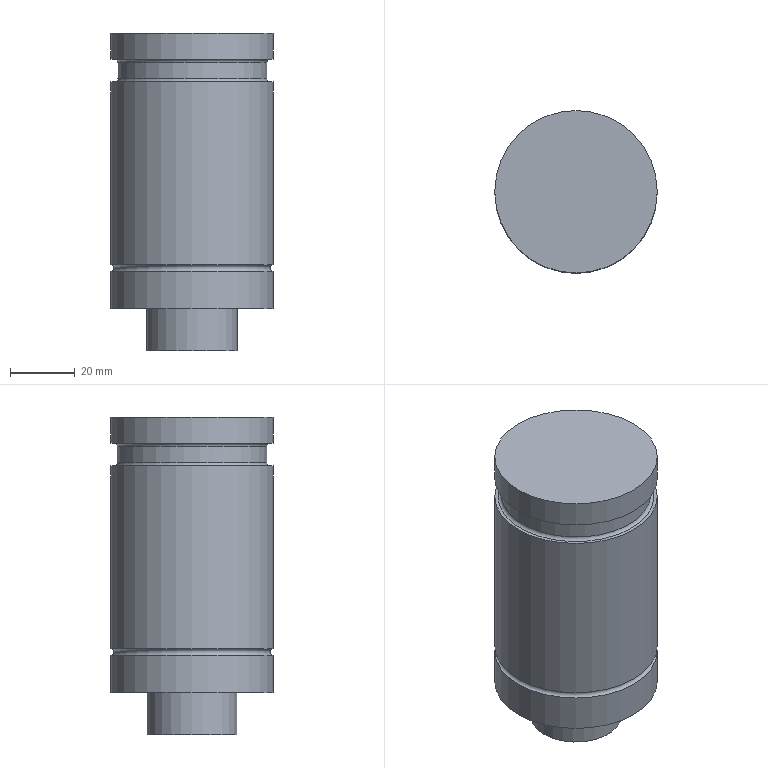Part | NX | features solid 2 | 1 solid | 13 faces | box 50.2 x 50.2 x 98 mm | volume 173939 mm3 | cylinder 5 | plane 5 | torus 3 | commonest cylinder face diameters 50.2 x3 28 x1 46.2 x1
STEP:
#1=CARTESIAN_POINT('',(40.1,-380.,248.5));
#2=VERTEX_POINT('',#1);
#3=CARTESIAN_POINT('',(15.,-380.,248.5));
#4=DIRECTION('',(0.,0.,1.));
#5=DIRECTION('',(1.,0.,0.));
#6=AXIS2_PLACEMENT_3D('',#3,#4,#5);
#7=CIRCLE('',#6,25.1);
#8=EDGE_CURVE('',#2,#2,#7,.T.);
#9=ORIENTED_EDGE('',*,*,#8,.T.);
#10=EDGE_LOOP('',(#9));
#11=FACE_BOUND('',#10,.T.);
#12=CARTESIAN_POINT('',(-10.1,-380.,305.));
#13=VERTEX_POINT('',#12);
#14=CARTESIAN_POINT('',(15.,-380.,305.));
#15=DIRECTION('',(0.,0.,-1.));
#16=DIRECTION('',(-1.,0.,0.));
#17=AXIS2_PLACEMENT_3D('',#14,#15,#16);
#18=CIRCLE('',#17,25.1);
#19=EDGE_CURVE('',#13,#13,#18,.T.);
#20=ORIENTED_EDGE('',*,*,#19,.T.);
#21=EDGE_LOOP('',(#20));
#22=FACE_BOUND('',#21,.T.);
#23=CARTESIAN_POINT('',(15.,-380.,235.));
#24=DIRECTION('',(0.,0.,1.));
#25=DIRECTION('',(1.,0.,0.));
#26=AXIS2_PLACEMENT_3D('',#23,#24,#25);
#27=CYLINDRICAL_SURFACE('',#26,25.1);
#28=ADVANCED_FACE('',(#11,#22),#27,.T.);
#29=CARTESIAN_POINT('',(1.,-380.,235.));
#30=VERTEX_POINT('',#29);
#31=CARTESIAN_POINT('',(15.,-380.,235.));
#32=DIRECTION('',(0.,0.,-1.));
#33=DIRECTION('',(-1.,0.,0.));
#34=AXIS2_PLACEMENT_3D('',#31,#32,#33);
#35=CIRCLE('',#34,14.);
#36=EDGE_CURVE('',#30,#30,#35,.T.);
#37=ORIENTED_EDGE('',*,*,#36,.F.);
#38=EDGE_LOOP('',(#37));
#39=FACE_BOUND('',#38,.T.);
#40=CARTESIAN_POINT('',(40.1,-380.,235.));
#41=VERTEX_POINT('',#40);
#42=CARTESIAN_POINT('',(15.,-380.,235.));
#43=DIRECTION('',(0.,0.,1.));
#44=DIRECTION('',(1.,0.,0.));
#45=AXIS2_PLACEMENT_3D('',#42,#43,#44);
#46=CIRCLE('',#45,25.1);
#47=EDGE_CURVE('',#41,#41,#46,.T.);
#48=ORIENTED_EDGE('',*,*,#47,.F.);
#49=EDGE_LOOP('',(#48));
#50=FACE_BOUND('',#49,.T.);
#51=CARTESIAN_POINT('',(15.,-380.,235.));
#52=DIRECTION('',(0.,0.,-1.));
#53=DIRECTION('',(-1.,0.,0.));
#54=AXIS2_PLACEMENT_3D('',#51,#52,#53);
#55=PLANE('',#54);
#56=ADVANCED_FACE('',(#39,#50),#55,.T.);
#57=CARTESIAN_POINT('',(40.1,-380.,246.5));
#58=VERTEX_POINT('',#57);
#59=CARTESIAN_POINT('',(15.,-380.,246.5));
#60=DIRECTION('',(0.,0.,1.));
#61=DIRECTION('',(1.,0.,0.));
#62=AXIS2_PLACEMENT_3D('',#59,#60,#61);
#63=CIRCLE('',#62,25.1);
#64=EDGE_CURVE('',#58,#58,#63,.T.);
#65=ORIENTED_EDGE('',*,*,#64,.F.);
#66=EDGE_LOOP('',(#65));
#67=FACE_BOUND('',#66,.T.);
#68=ORIENTED_EDGE('',*,*,#47,.T.);
#69=EDGE_LOOP('',(#68));
#70=FACE_BOUND('',#69,.T.);
#71=CARTESIAN_POINT('',(15.,-380.,235.));
#72=DIRECTION('',(0.,0.,1.));
#73=DIRECTION('',(1.,0.,0.));
#74=AXIS2_PLACEMENT_3D('',#71,#72,#73);
#75=CYLINDRICAL_SURFACE('',#74,25.1);
#76=ADVANCED_FACE('',(#67,#70),#75,.T.);
#77=CARTESIAN_POINT('',(29.,-380.,222.));
#78=VERTEX_POINT('',#77);
#79=CARTESIAN_POINT('',(15.,-380.,222.));
#80=DIRECTION('',(0.,0.,1.));
#81=DIRECTION('',(1.,0.,0.));
#82=AXIS2_PLACEMENT_3D('',#79,#80,#81);
#83=CIRCLE('',#82,14.);
#84=EDGE_CURVE('',#78,#78,#83,.T.);
#85=ORIENTED_EDGE('',*,*,#84,.F.);
#86=EDGE_LOOP('',(#85));
#87=FACE_BOUND('',#86,.T.);
#88=CARTESIAN_POINT('',(15.,-380.,222.));
#89=DIRECTION('',(0.,0.,-1.));
#90=DIRECTION('',(-1.,0.,0.));
#91=AXIS2_PLACEMENT_3D('',#88,#89,#90);
#92=PLANE('',#91);
#93=ADVANCED_FACE('',(#87),#92,.T.);
#94=ORIENTED_EDGE('',*,*,#84,.T.);
#95=EDGE_LOOP('',(#94));
#96=FACE_BOUND('',#95,.T.);
#97=ORIENTED_EDGE('',*,*,#36,.T.);
#98=EDGE_LOOP('',(#97));
#99=FACE_BOUND('',#98,.T.);
#100=CARTESIAN_POINT('',(15.,-380.,235.));
#101=DIRECTION('',(0.,0.,-1.));
#102=DIRECTION('',(-1.,0.,0.));
#103=AXIS2_PLACEMENT_3D('',#100,#101,#102);
#104=CYLINDRICAL_SURFACE('',#103,14.);
#105=ADVANCED_FACE('',(#96,#99),#104,.T.);
#106=ORIENTED_EDGE('',*,*,#8,.F.);
#107=EDGE_LOOP('',(#106));
#108=FACE_BOUND('',#107,.T.);
#109=ORIENTED_EDGE('',*,*,#64,.T.);
#110=EDGE_LOOP('',(#109));
#111=FACE_BOUND('',#110,.T.);
#112=CARTESIAN_POINT('',(15.,-380.,247.5));
#113=DIRECTION('',(0.,0.,-1.));
#114=DIRECTION('',(-1.,0.,0.));
#115=AXIS2_PLACEMENT_3D('',#112,#113,#114);
#116=TOROIDAL_SURFACE('',#115,25.1,1.);
#117=ADVANCED_FACE('',(#108,#111),#116,.F.);
#118=CARTESIAN_POINT('',(39.1,-380.,305.));
#119=VERTEX_POINT('',#118);
#120=CARTESIAN_POINT('',(15.,-380.,305.));
#121=DIRECTION('',(0.,0.,1.));
#122=DIRECTION('',(1.,0.,0.));
#123=AXIS2_PLACEMENT_3D('',#120,#121,#122);
#124=CIRCLE('',#123,24.1);
#125=EDGE_CURVE('',#119,#119,#124,.F.);
#126=ORIENTED_EDGE('',*,*,#125,.T.);
#127=EDGE_LOOP('',(#126));
#128=FACE_BOUND('',#127,.T.);
#129=ORIENTED_EDGE('',*,*,#19,.F.);
#130=EDGE_LOOP('',(#129));
#131=FACE_BOUND('',#130,.T.);
#132=CARTESIAN_POINT('',(15.,-380.,305.));
#133=DIRECTION('',(0.,0.,1.));
#134=DIRECTION('',(1.,0.,0.));
#135=AXIS2_PLACEMENT_3D('',#132,#133,#134);
#136=PLANE('',#135);
#137=ADVANCED_FACE('',(#128,#131),#136,.T.);
#138=CARTESIAN_POINT('',(39.1,-380.,312.));
#139=VERTEX_POINT('',#138);
#140=CARTESIAN_POINT('',(15.,-380.,312.));
#141=DIRECTION('',(0.,0.,1.));
#142=DIRECTION('',(1.,0.,0.));
#143=AXIS2_PLACEMENT_3D('',#140,#141,#142);
#144=CIRCLE('',#143,24.1);
#145=EDGE_CURVE('',#139,#139,#144,.T.);
#146=ORIENTED_EDGE('',*,*,#145,.T.);
#147=EDGE_LOOP('',(#146));
#148=FACE_BOUND('',#147,.T.);
#149=CARTESIAN_POINT('',(-10.1,-380.,312.));
#150=VERTEX_POINT('',#149);
#151=CARTESIAN_POINT('',(15.,-380.,312.));
#152=DIRECTION('',(0.,0.,-1.));
#153=DIRECTION('',(-1.,0.,0.));
#154=AXIS2_PLACEMENT_3D('',#151,#152,#153);
#155=CIRCLE('',#154,25.1);
#156=EDGE_CURVE('',#150,#150,#155,.T.);
#157=ORIENTED_EDGE('',*,*,#156,.T.);
#158=EDGE_LOOP('',(#157));
#159=FACE_BOUND('',#158,.T.);
#160=CARTESIAN_POINT('',(15.,-380.,312.));
#161=DIRECTION('',(0.,0.,1.));
#162=DIRECTION('',(1.,0.,0.));
#163=AXIS2_PLACEMENT_3D('',#160,#161,#162);
#164=PLANE('',#163);
#165=ADVANCED_FACE('',(#148,#159),#164,.F.);
#166=CARTESIAN_POINT('',(38.1,-380.,306.));
#167=VERTEX_POINT('',#166);
#168=CARTESIAN_POINT('',(15.,-380.,306.));
#169=DIRECTION('',(0.,0.,1.));
#170=DIRECTION('',(1.,0.,0.));
#171=AXIS2_PLACEMENT_3D('',#168,#169,#170);
#172=CIRCLE('',#171,23.1);
#173=EDGE_CURVE('',#167,#167,#172,.T.);
#174=ORIENTED_EDGE('',*,*,#173,.T.);
#175=EDGE_LOOP('',(#174));
#176=FACE_BOUND('',#175,.T.);
#177=CARTESIAN_POINT('',(38.1,-380.,311.));
#178=VERTEX_POINT('',#177);
#179=CARTESIAN_POINT('',(15.,-380.,311.));
#180=DIRECTION('',(0.,0.,1.));
#181=DIRECTION('',(1.,0.,0.));
#182=AXIS2_PLACEMENT_3D('',#179,#180,#181);
#183=CIRCLE('',#182,23.1);
#184=EDGE_CURVE('',#178,#178,#183,.F.);
#185=ORIENTED_EDGE('',*,*,#184,.T.);
#186=EDGE_LOOP('',(#185));
#187=FACE_BOUND('',#186,.T.);
#188=CARTESIAN_POINT('',(15.,-380.,312.));
#189=DIRECTION('',(0.,0.,-1.));
#190=DIRECTION('',(-1.,0.,0.));
#191=AXIS2_PLACEMENT_3D('',#188,#189,#190);
#192=CYLINDRICAL_SURFACE('',#191,23.1);
#193=ADVANCED_FACE('',(#176,#187),#192,.T.);
#194=CARTESIAN_POINT('',(-10.1,-380.,320.));
#195=VERTEX_POINT('',#194);
#196=CARTESIAN_POINT('',(15.,-380.,320.));
#197=DIRECTION('',(0.,0.,-1.));
#198=DIRECTION('',(-1.,0.,0.));
#199=AXIS2_PLACEMENT_3D('',#196,#197,#198);
#200=CIRCLE('',#199,25.1);
#201=EDGE_CURVE('',#195,#195,#200,.T.);
#202=ORIENTED_EDGE('',*,*,#201,.F.);
#203=EDGE_LOOP('',(#202));
#204=FACE_BOUND('',#203,.T.);
#205=CARTESIAN_POINT('',(15.,-380.,320.));
#206=DIRECTION('',(0.,0.,1.));
#207=DIRECTION('',(1.,0.,0.));
#208=AXIS2_PLACEMENT_3D('',#205,#206,#207);
#209=PLANE('',#208);
#210=ADVANCED_FACE('',(#204),#209,.T.);
#211=ORIENTED_EDGE('',*,*,#201,.T.);
#212=EDGE_LOOP('',(#211));
#213=FACE_BOUND('',#212,.T.);
#214=ORIENTED_EDGE('',*,*,#156,.F.);
#215=EDGE_LOOP('',(#214));
#216=FACE_BOUND('',#215,.T.);
#217=CARTESIAN_POINT('',(15.,-380.,235.));
#218=DIRECTION('',(0.,0.,1.));
#219=DIRECTION('',(1.,0.,0.));
#220=AXIS2_PLACEMENT_3D('',#217,#218,#219);
#221=CYLINDRICAL_SURFACE('',#220,25.1);
#222=ADVANCED_FACE('',(#213,#216),#221,.T.);
#223=ORIENTED_EDGE('',*,*,#173,.F.);
#224=EDGE_LOOP('',(#223));
#225=FACE_BOUND('',#224,.T.);
#226=ORIENTED_EDGE('',*,*,#125,.F.);
#227=EDGE_LOOP('',(#226));
#228=FACE_BOUND('',#227,.T.);
#229=CARTESIAN_POINT('',(15.,-380.,306.));
#230=DIRECTION('',(0.,0.,1.));
#231=DIRECTION('',(1.,0.,0.));
#232=AXIS2_PLACEMENT_3D('',#229,#230,#231);
#233=TOROIDAL_SURFACE('',#232,24.1,1.);
#234=ADVANCED_FACE('',(#225,#228),#233,.F.);
#235=ORIENTED_EDGE('',*,*,#145,.F.);
#236=EDGE_LOOP('',(#235));
#237=FACE_BOUND('',#236,.T.);
#238=ORIENTED_EDGE('',*,*,#184,.F.);
#239=EDGE_LOOP('',(#238));
#240=FACE_BOUND('',#239,.T.);
#241=CARTESIAN_POINT('',(15.,-380.,311.));
#242=DIRECTION('',(0.,0.,1.));
#243=DIRECTION('',(1.,0.,0.));
#244=AXIS2_PLACEMENT_3D('',#241,#242,#243);
#245=TOROIDAL_SURFACE('',#244,24.1,1.);
#246=ADVANCED_FACE('',(#237,#240),#245,.F.);
#247=CLOSED_SHELL('',(#28,#56,#76,#93,#105,#117,#137,#165,#193,#210,#222,#234,#246));
#248=MANIFOLD_SOLID_BREP('',#247);
#249=(LENGTH_UNIT()NAMED_UNIT(*)SI_UNIT(.MILLI.,.METRE.));
#250=UNCERTAINTY_MEASURE_WITH_UNIT(LENGTH_MEASURE(0.00001),#249,'','');
#251=(NAMED_UNIT(*)PLANE_ANGLE_UNIT()SI_UNIT($,.RADIAN.));
#252=(NAMED_UNIT(*)SI_UNIT($,.STERADIAN.)SOLID_ANGLE_UNIT());
#253=(GEOMETRIC_REPRESENTATION_CONTEXT(3)GLOBAL_UNCERTAINTY_ASSIGNED_CONTEXT((#250))GLOBAL_UNIT_ASSIGNED_CONTEXT((#249,#251,#252))REPRESENTATION_CONTEXT('',''));
#254=ADVANCED_BREP_SHAPE_REPRESENTATION('',(#248),#253);